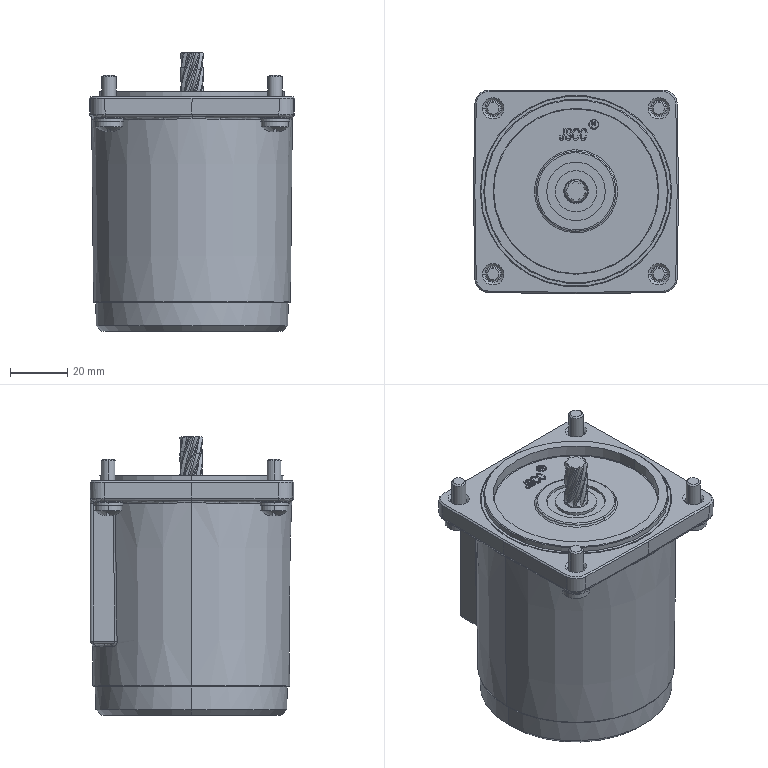Part | STEP file | QA-70YS15G | 2 solids | 588 faces | box 71.679 x 71.19 x 97.5 mm | volume 85810 mm3 | spline 228 | plane 205 | cylinder 106 | cone 49 | commonest cylinder face diameters 1 x16 2 x15 10 x12 5 x8 5.8 x8 9.5 x8